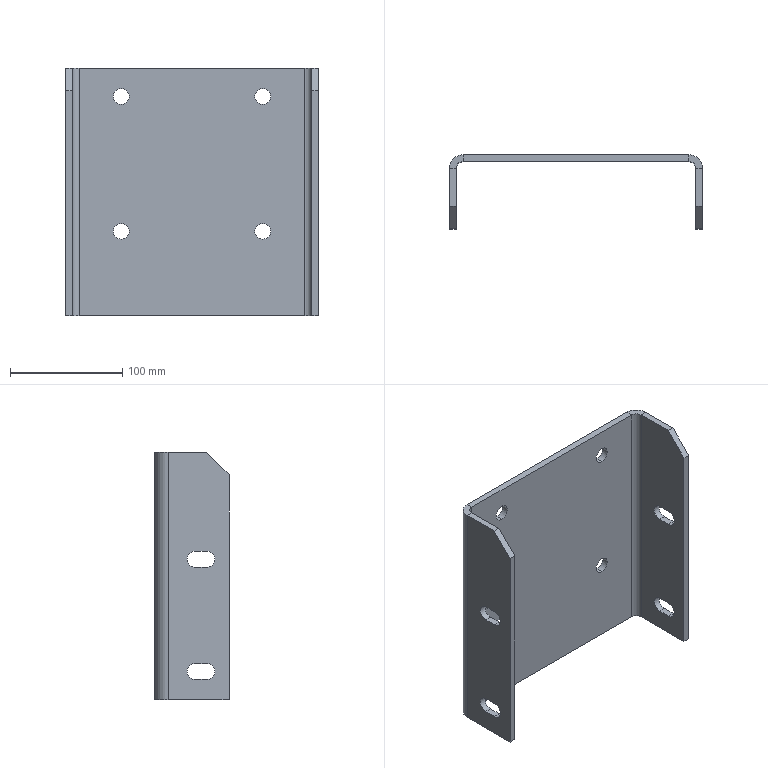Part | STEP file | Driven chain anti-jump bracket 1 | 1 solid | 48 faces | box 225 x 66 x 220 mm | volume 431717 mm3 | plane 28 | cylinder 20 | commonest cylinder face diameters 14 x16 12 x2 24 x2